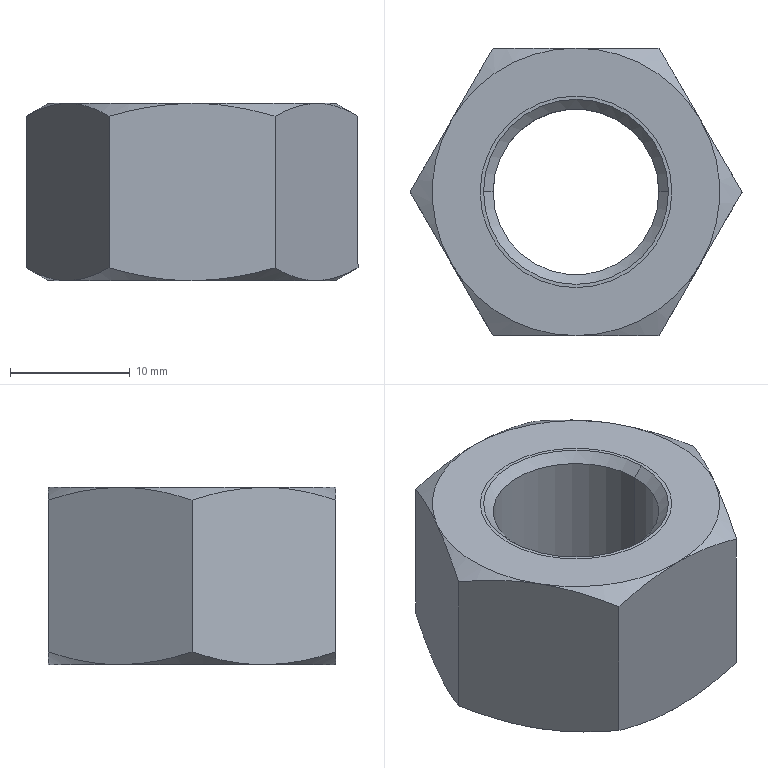Part | NX | features BREP 2 | 1 solid | 28 faces | box 27.713 x 24 x 14.8 mm | volume 7082 mm3 | cone 16 | plane 8 | cylinder 4 | commonest cylinder face diameters 13.835 x2 16 x2